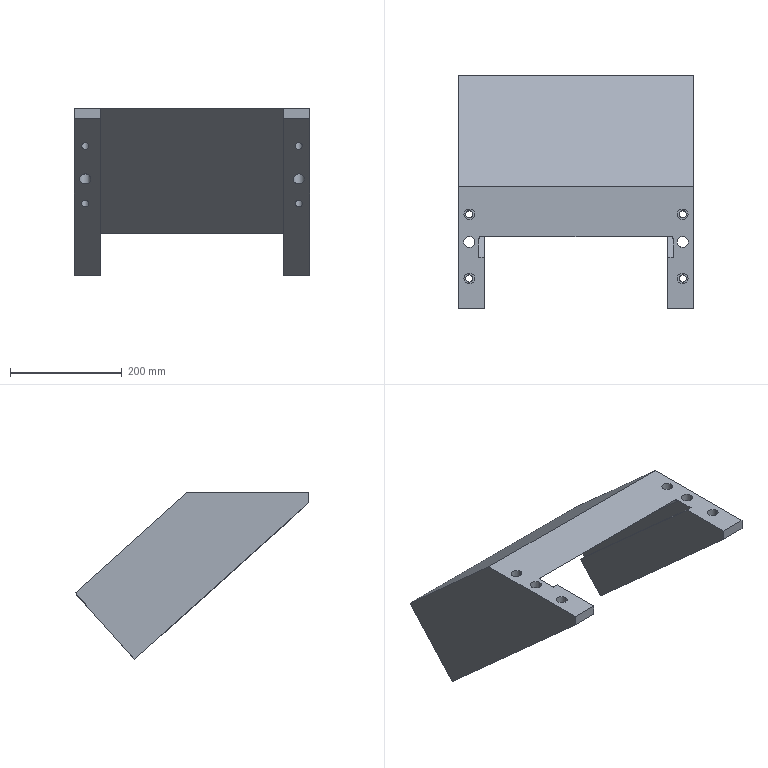Part | Creo | 1 solid | 66 faces | box 422.804 x 419.311 x 298.721 mm | volume 11000181 mm3 | cylinder 30 | plane 28 | cone 8 | commonest cylinder face diameters 8.782 x8 13 x8 19.25 x8 20 x4 8 x2